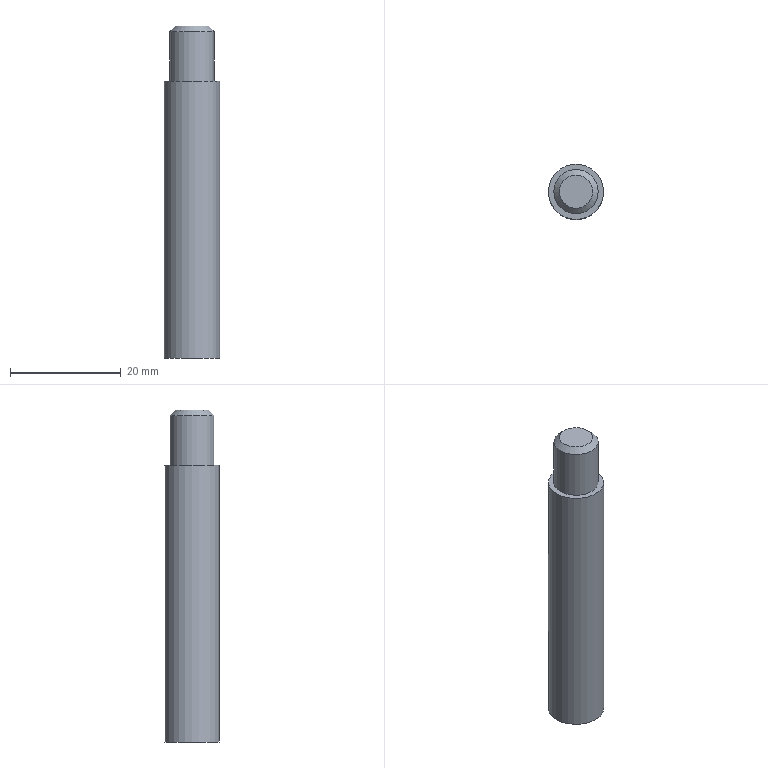Part | NX | features DATUM_CSYS 3, EXTRUDE 2, SKETCH 2, CHAMFER 1 | 1 solid | 6 faces | box 10 x 10 x 60 mm | volume 4418 mm3 | plane 3 | cylinder 2 | cone 1 | commonest cylinder face diameters 8 x1 10 x1
STEP:
#1=CARTESIAN_POINT('',(5.,0.,-50.));
#2=VERTEX_POINT('',#1);
#3=CARTESIAN_POINT('',(0.,0.,-50.));
#4=DIRECTION('',(0.,0.,1.));
#5=DIRECTION('',(1.,0.,0.));
#6=AXIS2_PLACEMENT_3D('',#3,#4,#5);
#7=CIRCLE('',#6,5.);
#8=EDGE_CURVE('',#2,#2,#7,.T.);
#9=ORIENTED_EDGE('',*,*,#8,.T.);
#10=EDGE_LOOP('',(#9));
#11=FACE_BOUND('',#10,.T.);
#12=CARTESIAN_POINT('',(5.,0.,0.));
#13=VERTEX_POINT('',#12);
#14=CARTESIAN_POINT('',(0.,0.,0.));
#15=DIRECTION('',(0.,0.,1.));
#16=DIRECTION('',(1.,0.,0.));
#17=AXIS2_PLACEMENT_3D('',#14,#15,#16);
#18=CIRCLE('',#17,5.);
#19=EDGE_CURVE('',#13,#13,#18,.T.);
#20=ORIENTED_EDGE('',*,*,#19,.F.);
#21=EDGE_LOOP('',(#20));
#22=FACE_BOUND('',#21,.T.);
#23=CARTESIAN_POINT('',(0.,0.,-50.));
#24=DIRECTION('',(0.,0.,1.));
#25=DIRECTION('',(1.,0.,0.));
#26=AXIS2_PLACEMENT_3D('',#23,#24,#25);
#27=CYLINDRICAL_SURFACE('',#26,5.);
#28=ADVANCED_FACE('',(#11,#22),#27,.T.);
#29=ORIENTED_EDGE('',*,*,#8,.F.);
#30=EDGE_LOOP('',(#29));
#31=FACE_BOUND('',#30,.T.);
#32=CARTESIAN_POINT('',(0.,0.,-50.));
#33=DIRECTION('',(0.,0.,1.));
#34=DIRECTION('',(1.,0.,0.));
#35=AXIS2_PLACEMENT_3D('',#32,#33,#34);
#36=PLANE('',#35);
#37=ADVANCED_FACE('',(#31),#36,.F.);
#38=CARTESIAN_POINT('',(4.,0.,0.));
#39=VERTEX_POINT('',#38);
#40=CARTESIAN_POINT('',(0.,0.,0.));
#41=DIRECTION('',(0.,0.,1.));
#42=DIRECTION('',(1.,0.,0.));
#43=AXIS2_PLACEMENT_3D('',#40,#41,#42);
#44=CIRCLE('',#43,4.);
#45=EDGE_CURVE('',#39,#39,#44,.T.);
#46=ORIENTED_EDGE('',*,*,#45,.F.);
#47=EDGE_LOOP('',(#46));
#48=FACE_BOUND('',#47,.T.);
#49=ORIENTED_EDGE('',*,*,#19,.T.);
#50=EDGE_LOOP('',(#49));
#51=FACE_BOUND('',#50,.T.);
#52=CARTESIAN_POINT('',(0.,0.,0.));
#53=DIRECTION('',(0.,0.,1.));
#54=DIRECTION('',(1.,0.,0.));
#55=AXIS2_PLACEMENT_3D('',#52,#53,#54);
#56=PLANE('',#55);
#57=ADVANCED_FACE('',(#48,#51),#56,.T.);
#58=CARTESIAN_POINT('',(4.,0.,9.));
#59=VERTEX_POINT('',#58);
#60=CARTESIAN_POINT('',(0.,0.,9.));
#61=DIRECTION('',(0.,0.,1.));
#62=DIRECTION('',(1.,0.,0.));
#63=AXIS2_PLACEMENT_3D('',#60,#61,#62);
#64=CIRCLE('',#63,4.);
#65=EDGE_CURVE('',#59,#59,#64,.F.);
#66=ORIENTED_EDGE('',*,*,#65,.T.);
#67=EDGE_LOOP('',(#66));
#68=FACE_BOUND('',#67,.T.);
#69=ORIENTED_EDGE('',*,*,#45,.T.);
#70=EDGE_LOOP('',(#69));
#71=FACE_BOUND('',#70,.T.);
#72=CARTESIAN_POINT('',(0.,0.,10.));
#73=DIRECTION('',(0.,0.,-1.));
#74=DIRECTION('',(-1.,0.,0.));
#75=AXIS2_PLACEMENT_3D('',#72,#73,#74);
#76=CYLINDRICAL_SURFACE('',#75,4.);
#77=ADVANCED_FACE('',(#68,#71),#76,.T.);
#78=CARTESIAN_POINT('',(3.,0.,10.));
#79=VERTEX_POINT('',#78);
#80=CARTESIAN_POINT('',(0.,0.,10.));
#81=DIRECTION('',(0.,0.,1.));
#82=DIRECTION('',(1.,0.,0.));
#83=AXIS2_PLACEMENT_3D('',#80,#81,#82);
#84=CIRCLE('',#83,3.);
#85=EDGE_CURVE('',#79,#79,#84,.T.);
#86=ORIENTED_EDGE('',*,*,#85,.T.);
#87=EDGE_LOOP('',(#86));
#88=FACE_BOUND('',#87,.T.);
#89=CARTESIAN_POINT('',(0.,0.,10.));
#90=DIRECTION('',(0.,0.,1.));
#91=DIRECTION('',(1.,0.,0.));
#92=AXIS2_PLACEMENT_3D('',#89,#90,#91);
#93=PLANE('',#92);
#94=ADVANCED_FACE('',(#88),#93,.T.);
#95=ORIENTED_EDGE('',*,*,#65,.F.);
#96=EDGE_LOOP('',(#95));
#97=FACE_BOUND('',#96,.T.);
#98=ORIENTED_EDGE('',*,*,#85,.F.);
#99=EDGE_LOOP('',(#98));
#100=FACE_BOUND('',#99,.T.);
#101=CARTESIAN_POINT('',(0.,0.,10.));
#102=DIRECTION('',(0.,0.,-1.));
#103=DIRECTION('',(-1.,0.,0.));
#104=AXIS2_PLACEMENT_3D('',#101,#102,#103);
#105=CONICAL_SURFACE('',#104,3.,0.7854);
#106=ADVANCED_FACE('',(#97,#100),#105,.T.);
#107=CLOSED_SHELL('',(#28,#37,#57,#77,#94,#106));
#108=MANIFOLD_SOLID_BREP('',#107);
#109=(LENGTH_UNIT()NAMED_UNIT(*)SI_UNIT(.MILLI.,.METRE.));
#110=UNCERTAINTY_MEASURE_WITH_UNIT(LENGTH_MEASURE(0.00001),#109,'','');
#111=(NAMED_UNIT(*)PLANE_ANGLE_UNIT()SI_UNIT($,.RADIAN.));
#112=(NAMED_UNIT(*)SI_UNIT($,.STERADIAN.)SOLID_ANGLE_UNIT());
#113=(GEOMETRIC_REPRESENTATION_CONTEXT(3)GLOBAL_UNCERTAINTY_ASSIGNED_CONTEXT((#110))GLOBAL_UNIT_ASSIGNED_CONTEXT((#109,#111,#112))REPRESENTATION_CONTEXT('',''));
#114=ADVANCED_BREP_SHAPE_REPRESENTATION('',(#108),#113);